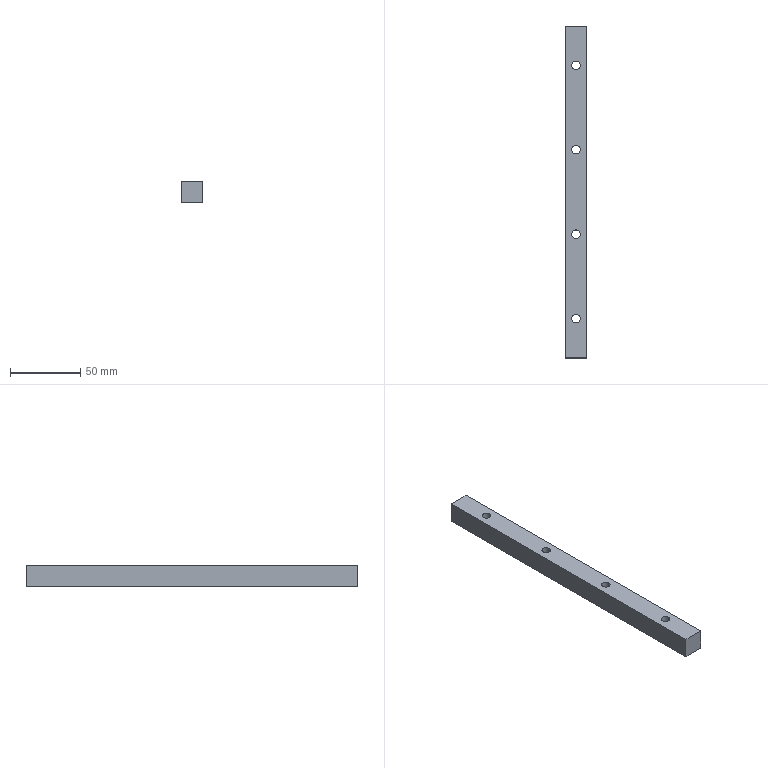Part | 1 solid | 14 faces | box 15 x 236 x 15 mm | volume 51404 mm3 | cylinder 8 | plane 6 | commonest cylinder face diameters 6 x8
STEP:
#1=CARTESIAN_POINT('',(-3.,208.,-7.5));
#2=VERTEX_POINT('',#1);
#3=CARTESIAN_POINT('',(3.,208.,-7.5));
#4=VERTEX_POINT('',#3);
#5=CARTESIAN_POINT('',(0.,208.,-7.5));
#6=DIRECTION('',(0.,0.,1.));
#7=DIRECTION('',(1.,0.,0.));
#8=AXIS2_PLACEMENT_3D('',#5,#6,#7);
#9=CIRCLE('',#8,3.);
#10=EDGE_CURVE('',#2,#4,#9,.T.);
#11=ORIENTED_EDGE('',*,*,#10,.F.);
#12=CARTESIAN_POINT('',(-3.,208.,7.5));
#13=VERTEX_POINT('',#12);
#14=CARTESIAN_POINT('',(-3.,208.,7.5));
#15=DIRECTION('',(0.,0.,1.));
#16=VECTOR('',#15,1000.);
#17=LINE('',#14,#16);
#18=EDGE_CURVE('',#2,#13,#17,.T.);
#19=ORIENTED_EDGE('',*,*,#18,.T.);
#20=CARTESIAN_POINT('',(3.,208.,7.5));
#21=VERTEX_POINT('',#20);
#22=CARTESIAN_POINT('',(0.,208.,7.5));
#23=DIRECTION('',(0.,0.,1.));
#24=DIRECTION('',(1.,0.,0.));
#25=AXIS2_PLACEMENT_3D('',#22,#23,#24);
#26=CIRCLE('',#25,3.);
#27=EDGE_CURVE('',#13,#21,#26,.T.);
#28=ORIENTED_EDGE('',*,*,#27,.T.);
#29=CARTESIAN_POINT('',(3.,208.,7.5));
#30=DIRECTION('',(0.,0.,1.));
#31=VECTOR('',#30,1000.);
#32=LINE('',#29,#31);
#33=EDGE_CURVE('',#4,#21,#32,.T.);
#34=ORIENTED_EDGE('',*,*,#33,.F.);
#35=EDGE_LOOP('',(#11,#19,#28,#34));
#36=FACE_OUTER_BOUND('',#35,.T.);
#37=CARTESIAN_POINT('',(0.,208.,7.5));
#38=DIRECTION('',(0.,0.,1.));
#39=DIRECTION('',(1.,0.,0.));
#40=AXIS2_PLACEMENT_3D('',#37,#38,#39);
#41=CYLINDRICAL_SURFACE('',#40,3.);
#42=ADVANCED_FACE('',(#36),#41,.F.);
#43=CARTESIAN_POINT('',(-3.,148.,-7.5));
#44=VERTEX_POINT('',#43);
#45=CARTESIAN_POINT('',(3.,148.,-7.5));
#46=VERTEX_POINT('',#45);
#47=CARTESIAN_POINT('',(0.,148.,-7.5));
#48=DIRECTION('',(0.,0.,1.));
#49=DIRECTION('',(1.,0.,0.));
#50=AXIS2_PLACEMENT_3D('',#47,#48,#49);
#51=CIRCLE('',#50,3.);
#52=EDGE_CURVE('',#44,#46,#51,.T.);
#53=ORIENTED_EDGE('',*,*,#52,.F.);
#54=CARTESIAN_POINT('',(-3.,148.,7.5));
#55=VERTEX_POINT('',#54);
#56=CARTESIAN_POINT('',(-3.,148.,7.5));
#57=DIRECTION('',(0.,0.,1.));
#58=VECTOR('',#57,1000.);
#59=LINE('',#56,#58);
#60=EDGE_CURVE('',#44,#55,#59,.T.);
#61=ORIENTED_EDGE('',*,*,#60,.T.);
#62=CARTESIAN_POINT('',(3.,148.,7.5));
#63=VERTEX_POINT('',#62);
#64=CARTESIAN_POINT('',(0.,148.,7.5));
#65=DIRECTION('',(0.,0.,1.));
#66=DIRECTION('',(1.,0.,0.));
#67=AXIS2_PLACEMENT_3D('',#64,#65,#66);
#68=CIRCLE('',#67,3.);
#69=EDGE_CURVE('',#55,#63,#68,.T.);
#70=ORIENTED_EDGE('',*,*,#69,.T.);
#71=CARTESIAN_POINT('',(3.,148.,7.5));
#72=DIRECTION('',(0.,0.,1.));
#73=VECTOR('',#72,1000.);
#74=LINE('',#71,#73);
#75=EDGE_CURVE('',#46,#63,#74,.T.);
#76=ORIENTED_EDGE('',*,*,#75,.F.);
#77=EDGE_LOOP('',(#53,#61,#70,#76));
#78=FACE_OUTER_BOUND('',#77,.T.);
#79=CARTESIAN_POINT('',(0.,148.,7.5));
#80=DIRECTION('',(0.,0.,1.));
#81=DIRECTION('',(1.,0.,0.));
#82=AXIS2_PLACEMENT_3D('',#79,#80,#81);
#83=CYLINDRICAL_SURFACE('',#82,3.);
#84=ADVANCED_FACE('',(#78),#83,.F.);
#85=CARTESIAN_POINT('',(-3.,88.,-7.5));
#86=VERTEX_POINT('',#85);
#87=CARTESIAN_POINT('',(3.,88.,-7.5));
#88=VERTEX_POINT('',#87);
#89=CARTESIAN_POINT('',(0.,88.,-7.5));
#90=DIRECTION('',(0.,0.,1.));
#91=DIRECTION('',(1.,0.,0.));
#92=AXIS2_PLACEMENT_3D('',#89,#90,#91);
#93=CIRCLE('',#92,3.);
#94=EDGE_CURVE('',#86,#88,#93,.T.);
#95=ORIENTED_EDGE('',*,*,#94,.F.);
#96=CARTESIAN_POINT('',(-3.,88.,7.5));
#97=VERTEX_POINT('',#96);
#98=CARTESIAN_POINT('',(-3.,88.,7.5));
#99=DIRECTION('',(0.,0.,1.));
#100=VECTOR('',#99,1000.);
#101=LINE('',#98,#100);
#102=EDGE_CURVE('',#86,#97,#101,.T.);
#103=ORIENTED_EDGE('',*,*,#102,.T.);
#104=CARTESIAN_POINT('',(3.,88.,7.5));
#105=VERTEX_POINT('',#104);
#106=CARTESIAN_POINT('',(0.,88.,7.5));
#107=DIRECTION('',(0.,0.,1.));
#108=DIRECTION('',(1.,0.,0.));
#109=AXIS2_PLACEMENT_3D('',#106,#107,#108);
#110=CIRCLE('',#109,3.);
#111=EDGE_CURVE('',#97,#105,#110,.T.);
#112=ORIENTED_EDGE('',*,*,#111,.T.);
#113=CARTESIAN_POINT('',(3.,88.,7.5));
#114=DIRECTION('',(0.,0.,1.));
#115=VECTOR('',#114,1000.);
#116=LINE('',#113,#115);
#117=EDGE_CURVE('',#88,#105,#116,.T.);
#118=ORIENTED_EDGE('',*,*,#117,.F.);
#119=EDGE_LOOP('',(#95,#103,#112,#118));
#120=FACE_OUTER_BOUND('',#119,.T.);
#121=CARTESIAN_POINT('',(0.,88.,7.5));
#122=DIRECTION('',(0.,0.,1.));
#123=DIRECTION('',(1.,0.,0.));
#124=AXIS2_PLACEMENT_3D('',#121,#122,#123);
#125=CYLINDRICAL_SURFACE('',#124,3.);
#126=ADVANCED_FACE('',(#120),#125,.F.);
#127=CARTESIAN_POINT('',(-3.,28.,-7.5));
#128=VERTEX_POINT('',#127);
#129=CARTESIAN_POINT('',(3.,28.,-7.5));
#130=VERTEX_POINT('',#129);
#131=CARTESIAN_POINT('',(0.,28.,-7.5));
#132=DIRECTION('',(0.,0.,1.));
#133=DIRECTION('',(1.,0.,0.));
#134=AXIS2_PLACEMENT_3D('',#131,#132,#133);
#135=CIRCLE('',#134,3.);
#136=EDGE_CURVE('',#128,#130,#135,.T.);
#137=ORIENTED_EDGE('',*,*,#136,.F.);
#138=CARTESIAN_POINT('',(-3.,28.,7.5));
#139=VERTEX_POINT('',#138);
#140=CARTESIAN_POINT('',(-3.,28.,7.5));
#141=DIRECTION('',(0.,0.,1.));
#142=VECTOR('',#141,1000.);
#143=LINE('',#140,#142);
#144=EDGE_CURVE('',#128,#139,#143,.T.);
#145=ORIENTED_EDGE('',*,*,#144,.T.);
#146=CARTESIAN_POINT('',(3.,28.,7.5));
#147=VERTEX_POINT('',#146);
#148=CARTESIAN_POINT('',(0.,28.,7.5));
#149=DIRECTION('',(0.,0.,1.));
#150=DIRECTION('',(1.,0.,0.));
#151=AXIS2_PLACEMENT_3D('',#148,#149,#150);
#152=CIRCLE('',#151,3.);
#153=EDGE_CURVE('',#139,#147,#152,.T.);
#154=ORIENTED_EDGE('',*,*,#153,.T.);
#155=CARTESIAN_POINT('',(3.,28.,7.5));
#156=DIRECTION('',(0.,0.,1.));
#157=VECTOR('',#156,1000.);
#158=LINE('',#155,#157);
#159=EDGE_CURVE('',#130,#147,#158,.T.);
#160=ORIENTED_EDGE('',*,*,#159,.F.);
#161=EDGE_LOOP('',(#137,#145,#154,#160));
#162=FACE_OUTER_BOUND('',#161,.T.);
#163=CARTESIAN_POINT('',(0.,28.,7.5));
#164=DIRECTION('',(0.,0.,1.));
#165=DIRECTION('',(1.,0.,0.));
#166=AXIS2_PLACEMENT_3D('',#163,#164,#165);
#167=CYLINDRICAL_SURFACE('',#166,3.);
#168=ADVANCED_FACE('',(#162),#167,.F.);
#169=CARTESIAN_POINT('',(0.,208.,7.5));
#170=DIRECTION('',(0.,0.,1.));
#171=DIRECTION('',(1.,0.,0.));
#172=AXIS2_PLACEMENT_3D('',#169,#170,#171);
#173=CIRCLE('',#172,3.);
#174=EDGE_CURVE('',#21,#13,#173,.T.);
#175=ORIENTED_EDGE('',*,*,#174,.F.);
#176=ORIENTED_EDGE('',*,*,#27,.F.);
#177=EDGE_LOOP('',(#175,#176));
#178=FACE_BOUND('',#177,.T.);
#179=CARTESIAN_POINT('',(0.,148.,7.5));
#180=DIRECTION('',(0.,0.,1.));
#181=DIRECTION('',(1.,0.,0.));
#182=AXIS2_PLACEMENT_3D('',#179,#180,#181);
#183=CIRCLE('',#182,3.);
#184=EDGE_CURVE('',#63,#55,#183,.T.);
#185=ORIENTED_EDGE('',*,*,#184,.F.);
#186=ORIENTED_EDGE('',*,*,#69,.F.);
#187=EDGE_LOOP('',(#185,#186));
#188=FACE_BOUND('',#187,.T.);
#189=CARTESIAN_POINT('',(0.,88.,7.5));
#190=DIRECTION('',(0.,0.,1.));
#191=DIRECTION('',(1.,0.,0.));
#192=AXIS2_PLACEMENT_3D('',#189,#190,#191);
#193=CIRCLE('',#192,3.);
#194=EDGE_CURVE('',#105,#97,#193,.T.);
#195=ORIENTED_EDGE('',*,*,#194,.F.);
#196=ORIENTED_EDGE('',*,*,#111,.F.);
#197=EDGE_LOOP('',(#195,#196));
#198=FACE_BOUND('',#197,.T.);
#199=CARTESIAN_POINT('',(-7.5,0.,7.5));
#200=VERTEX_POINT('',#199);
#201=CARTESIAN_POINT('',(7.5,0.,7.5));
#202=VERTEX_POINT('',#201);
#203=CARTESIAN_POINT('',(-7.5,0.,7.5));
#204=DIRECTION('',(1.,0.,0.));
#205=VECTOR('',#204,1000.);
#206=LINE('',#203,#205);
#207=EDGE_CURVE('',#200,#202,#206,.T.);
#208=ORIENTED_EDGE('',*,*,#207,.T.);
#209=CARTESIAN_POINT('',(7.5,236.,7.5));
#210=VERTEX_POINT('',#209);
#211=CARTESIAN_POINT('',(7.5,236.,7.5));
#212=DIRECTION('',(0.,-1.,0.));
#213=VECTOR('',#212,1000.);
#214=LINE('',#211,#213);
#215=EDGE_CURVE('',#210,#202,#214,.T.);
#216=ORIENTED_EDGE('',*,*,#215,.F.);
#217=CARTESIAN_POINT('',(-7.5,236.,7.5));
#218=VERTEX_POINT('',#217);
#219=CARTESIAN_POINT('',(-7.5,236.,7.5));
#220=DIRECTION('',(1.,0.,0.));
#221=VECTOR('',#220,1000.);
#222=LINE('',#219,#221);
#223=EDGE_CURVE('',#218,#210,#222,.T.);
#224=ORIENTED_EDGE('',*,*,#223,.F.);
#225=CARTESIAN_POINT('',(-7.5,236.,7.5));
#226=DIRECTION('',(0.,-1.,0.));
#227=VECTOR('',#226,1000.);
#228=LINE('',#225,#227);
#229=EDGE_CURVE('',#218,#200,#228,.T.);
#230=ORIENTED_EDGE('',*,*,#229,.T.);
#231=EDGE_LOOP('',(#208,#216,#224,#230));
#232=FACE_OUTER_BOUND('',#231,.T.);
#233=CARTESIAN_POINT('',(0.,28.,7.5));
#234=DIRECTION('',(0.,0.,1.));
#235=DIRECTION('',(1.,0.,0.));
#236=AXIS2_PLACEMENT_3D('',#233,#234,#235);
#237=CIRCLE('',#236,3.);
#238=EDGE_CURVE('',#147,#139,#237,.T.);
#239=ORIENTED_EDGE('',*,*,#238,.F.);
#240=ORIENTED_EDGE('',*,*,#153,.F.);
#241=EDGE_LOOP('',(#239,#240));
#242=FACE_BOUND('',#241,.T.);
#243=CARTESIAN_POINT('',(-7.5,236.,7.5));
#244=DIRECTION('',(0.,0.,-1.));
#245=DIRECTION('',(-1.,0.,0.));
#246=AXIS2_PLACEMENT_3D('',#243,#244,#245);
#247=PLANE('',#246);
#248=ADVANCED_FACE('',(#178,#188,#198,#232,#242),#247,.F.);
#249=CARTESIAN_POINT('',(7.5,0.,-7.5));
#250=VERTEX_POINT('',#249);
#251=CARTESIAN_POINT('',(7.5,0.,7.5));
#252=DIRECTION('',(0.,0.,-1.));
#253=VECTOR('',#252,1000.);
#254=LINE('',#251,#253);
#255=EDGE_CURVE('',#202,#250,#254,.T.);
#256=ORIENTED_EDGE('',*,*,#255,.T.);
#257=CARTESIAN_POINT('',(7.5,236.,-7.5));
#258=VERTEX_POINT('',#257);
#259=CARTESIAN_POINT('',(7.5,236.,-7.5));
#260=DIRECTION('',(0.,-1.,0.));
#261=VECTOR('',#260,1000.);
#262=LINE('',#259,#261);
#263=EDGE_CURVE('',#258,#250,#262,.T.);
#264=ORIENTED_EDGE('',*,*,#263,.F.);
#265=CARTESIAN_POINT('',(7.5,236.,7.5));
#266=DIRECTION('',(0.,0.,-1.));
#267=VECTOR('',#266,1000.);
#268=LINE('',#265,#267);
#269=EDGE_CURVE('',#210,#258,#268,.T.);
#270=ORIENTED_EDGE('',*,*,#269,.F.);
#271=ORIENTED_EDGE('',*,*,#215,.T.);
#272=EDGE_LOOP('',(#256,#264,#270,#271));
#273=FACE_OUTER_BOUND('',#272,.T.);
#274=CARTESIAN_POINT('',(7.5,236.,7.5));
#275=DIRECTION('',(-1.,0.,0.));
#276=DIRECTION('',(0.,0.,1.));
#277=AXIS2_PLACEMENT_3D('',#274,#275,#276);
#278=PLANE('',#277);
#279=ADVANCED_FACE('',(#273),#278,.F.);
#280=CARTESIAN_POINT('',(0.,208.,-7.5));
#281=DIRECTION('',(0.,0.,1.));
#282=DIRECTION('',(1.,0.,0.));
#283=AXIS2_PLACEMENT_3D('',#280,#281,#282);
#284=CIRCLE('',#283,3.);
#285=EDGE_CURVE('',#4,#2,#284,.T.);
#286=ORIENTED_EDGE('',*,*,#285,.T.);
#287=ORIENTED_EDGE('',*,*,#10,.T.);
#288=EDGE_LOOP('',(#286,#287));
#289=FACE_BOUND('',#288,.T.);
#290=CARTESIAN_POINT('',(0.,148.,-7.5));
#291=DIRECTION('',(0.,0.,1.));
#292=DIRECTION('',(1.,0.,0.));
#293=AXIS2_PLACEMENT_3D('',#290,#291,#292);
#294=CIRCLE('',#293,3.);
#295=EDGE_CURVE('',#46,#44,#294,.T.);
#296=ORIENTED_EDGE('',*,*,#295,.T.);
#297=ORIENTED_EDGE('',*,*,#52,.T.);
#298=EDGE_LOOP('',(#296,#297));
#299=FACE_BOUND('',#298,.T.);
#300=CARTESIAN_POINT('',(0.,88.,-7.5));
#301=DIRECTION('',(0.,0.,1.));
#302=DIRECTION('',(1.,0.,0.));
#303=AXIS2_PLACEMENT_3D('',#300,#301,#302);
#304=CIRCLE('',#303,3.);
#305=EDGE_CURVE('',#88,#86,#304,.T.);
#306=ORIENTED_EDGE('',*,*,#305,.T.);
#307=ORIENTED_EDGE('',*,*,#94,.T.);
#308=EDGE_LOOP('',(#306,#307));
#309=FACE_BOUND('',#308,.T.);
#310=CARTESIAN_POINT('',(0.,28.,-7.5));
#311=DIRECTION('',(0.,0.,1.));
#312=DIRECTION('',(1.,0.,0.));
#313=AXIS2_PLACEMENT_3D('',#310,#311,#312);
#314=CIRCLE('',#313,3.);
#315=EDGE_CURVE('',#130,#128,#314,.T.);
#316=ORIENTED_EDGE('',*,*,#315,.T.);
#317=ORIENTED_EDGE('',*,*,#136,.T.);
#318=EDGE_LOOP('',(#316,#317));
#319=FACE_BOUND('',#318,.T.);
#320=CARTESIAN_POINT('',(-7.5,0.,-7.5));
#321=VERTEX_POINT('',#320);
#322=CARTESIAN_POINT('',(-7.5,0.,-7.5));
#323=DIRECTION('',(-1.,0.,0.));
#324=VECTOR('',#323,1000.);
#325=LINE('',#322,#324);
#326=EDGE_CURVE('',#250,#321,#325,.T.);
#327=ORIENTED_EDGE('',*,*,#326,.T.);
#328=CARTESIAN_POINT('',(-7.5,236.,-7.5));
#329=VERTEX_POINT('',#328);
#330=CARTESIAN_POINT('',(-7.5,236.,-7.5));
#331=DIRECTION('',(0.,-1.,0.));
#332=VECTOR('',#331,1000.);
#333=LINE('',#330,#332);
#334=EDGE_CURVE('',#329,#321,#333,.T.);
#335=ORIENTED_EDGE('',*,*,#334,.F.);
#336=CARTESIAN_POINT('',(-7.5,236.,-7.5));
#337=DIRECTION('',(-1.,0.,0.));
#338=VECTOR('',#337,1000.);
#339=LINE('',#336,#338);
#340=EDGE_CURVE('',#258,#329,#339,.T.);
#341=ORIENTED_EDGE('',*,*,#340,.F.);
#342=ORIENTED_EDGE('',*,*,#263,.T.);
#343=EDGE_LOOP('',(#327,#335,#341,#342));
#344=FACE_OUTER_BOUND('',#343,.T.);
#345=CARTESIAN_POINT('',(-7.5,236.,-7.5));
#346=DIRECTION('',(0.,0.,1.));
#347=DIRECTION('',(1.,0.,0.));
#348=AXIS2_PLACEMENT_3D('',#345,#346,#347);
#349=PLANE('',#348);
#350=ADVANCED_FACE('',(#289,#299,#309,#319,#344),#349,.F.);
#351=CARTESIAN_POINT('',(-7.5,0.,7.5));
#352=DIRECTION('',(0.,0.,1.));
#353=VECTOR('',#352,1000.);
#354=LINE('',#351,#353);
#355=EDGE_CURVE('',#321,#200,#354,.T.);
#356=ORIENTED_EDGE('',*,*,#355,.T.);
#357=ORIENTED_EDGE('',*,*,#229,.F.);
#358=CARTESIAN_POINT('',(-7.5,236.,7.5));
#359=DIRECTION('',(0.,0.,1.));
#360=VECTOR('',#359,1000.);
#361=LINE('',#358,#360);
#362=EDGE_CURVE('',#329,#218,#361,.T.);
#363=ORIENTED_EDGE('',*,*,#362,.F.);
#364=ORIENTED_EDGE('',*,*,#334,.T.);
#365=EDGE_LOOP('',(#356,#357,#363,#364));
#366=FACE_OUTER_BOUND('',#365,.T.);
#367=CARTESIAN_POINT('',(-7.5,236.,7.5));
#368=DIRECTION('',(1.,0.,0.));
#369=DIRECTION('',(0.,0.,-1.));
#370=AXIS2_PLACEMENT_3D('',#367,#368,#369);
#371=PLANE('',#370);
#372=ADVANCED_FACE('',(#366),#371,.F.);
#373=ORIENTED_EDGE('',*,*,#269,.T.);
#374=ORIENTED_EDGE('',*,*,#340,.T.);
#375=ORIENTED_EDGE('',*,*,#362,.T.);
#376=ORIENTED_EDGE('',*,*,#223,.T.);
#377=EDGE_LOOP('',(#373,#374,#375,#376));
#378=FACE_OUTER_BOUND('',#377,.T.);
#379=CARTESIAN_POINT('',(0.,236.,0.));
#380=DIRECTION('',(0.,-1.,0.));
#381=DIRECTION('',(0.,0.,-1.));
#382=AXIS2_PLACEMENT_3D('',#379,#380,#381);
#383=PLANE('',#382);
#384=ADVANCED_FACE('',(#378),#383,.F.);
#385=ORIENTED_EDGE('',*,*,#255,.F.);
#386=ORIENTED_EDGE('',*,*,#207,.F.);
#387=ORIENTED_EDGE('',*,*,#355,.F.);
#388=ORIENTED_EDGE('',*,*,#326,.F.);
#389=EDGE_LOOP('',(#385,#386,#387,#388));
#390=FACE_OUTER_BOUND('',#389,.T.);
#391=CARTESIAN_POINT('',(0.,0.,0.));
#392=DIRECTION('',(0.,-1.,0.));
#393=DIRECTION('',(0.,0.,-1.));
#394=AXIS2_PLACEMENT_3D('',#391,#392,#393);
#395=PLANE('',#394);
#396=ADVANCED_FACE('',(#390),#395,.T.);
#397=ORIENTED_EDGE('',*,*,#144,.F.);
#398=ORIENTED_EDGE('',*,*,#315,.F.);
#399=ORIENTED_EDGE('',*,*,#159,.T.);
#400=ORIENTED_EDGE('',*,*,#238,.T.);
#401=EDGE_LOOP('',(#397,#398,#399,#400));
#402=FACE_OUTER_BOUND('',#401,.T.);
#403=CARTESIAN_POINT('',(0.,28.,7.5));
#404=DIRECTION('',(0.,0.,1.));
#405=DIRECTION('',(1.,0.,0.));
#406=AXIS2_PLACEMENT_3D('',#403,#404,#405);
#407=CYLINDRICAL_SURFACE('',#406,3.);
#408=ADVANCED_FACE('',(#402),#407,.F.);
#409=ORIENTED_EDGE('',*,*,#102,.F.);
#410=ORIENTED_EDGE('',*,*,#305,.F.);
#411=ORIENTED_EDGE('',*,*,#117,.T.);
#412=ORIENTED_EDGE('',*,*,#194,.T.);
#413=EDGE_LOOP('',(#409,#410,#411,#412));
#414=FACE_OUTER_BOUND('',#413,.T.);
#415=CARTESIAN_POINT('',(0.,88.,7.5));
#416=DIRECTION('',(0.,0.,1.));
#417=DIRECTION('',(1.,0.,0.));
#418=AXIS2_PLACEMENT_3D('',#415,#416,#417);
#419=CYLINDRICAL_SURFACE('',#418,3.);
#420=ADVANCED_FACE('',(#414),#419,.F.);
#421=ORIENTED_EDGE('',*,*,#60,.F.);
#422=ORIENTED_EDGE('',*,*,#295,.F.);
#423=ORIENTED_EDGE('',*,*,#75,.T.);
#424=ORIENTED_EDGE('',*,*,#184,.T.);
#425=EDGE_LOOP('',(#421,#422,#423,#424));
#426=FACE_OUTER_BOUND('',#425,.T.);
#427=CARTESIAN_POINT('',(0.,148.,7.5));
#428=DIRECTION('',(0.,0.,1.));
#429=DIRECTION('',(1.,0.,0.));
#430=AXIS2_PLACEMENT_3D('',#427,#428,#429);
#431=CYLINDRICAL_SURFACE('',#430,3.);
#432=ADVANCED_FACE('',(#426),#431,.F.);
#433=ORIENTED_EDGE('',*,*,#18,.F.);
#434=ORIENTED_EDGE('',*,*,#285,.F.);
#435=ORIENTED_EDGE('',*,*,#33,.T.);
#436=ORIENTED_EDGE('',*,*,#174,.T.);
#437=EDGE_LOOP('',(#433,#434,#435,#436));
#438=FACE_OUTER_BOUND('',#437,.T.);
#439=CARTESIAN_POINT('',(0.,208.,7.5));
#440=DIRECTION('',(0.,0.,1.));
#441=DIRECTION('',(1.,0.,0.));
#442=AXIS2_PLACEMENT_3D('',#439,#440,#441);
#443=CYLINDRICAL_SURFACE('',#442,3.);
#444=ADVANCED_FACE('',(#438),#443,.F.);
#445=CLOSED_SHELL('',(#42,#84,#126,#168,#248,#279,#350,#372,#384,#396,#408,#420,#432,#444));
#446=MANIFOLD_SOLID_BREP('',#445);
#447=CARTESIAN_POINT('',(0.,0.,0.));
#448=DIRECTION('',(0.,0.,1.));
#449=DIRECTION('',(1.,0.,0.));
#450=AXIS2_PLACEMENT_3D('',#447,#448,#449);
#451=(LENGTH_UNIT()NAMED_UNIT(*)SI_UNIT(.MILLI.,.METRE.));
#452=UNCERTAINTY_MEASURE_WITH_UNIT(LENGTH_MEASURE(0.00001),#451,'','');
#453=(NAMED_UNIT(*)PLANE_ANGLE_UNIT()SI_UNIT($,.RADIAN.));
#454=(NAMED_UNIT(*)SI_UNIT($,.STERADIAN.)SOLID_ANGLE_UNIT());
#455=(GEOMETRIC_REPRESENTATION_CONTEXT(3)GLOBAL_UNCERTAINTY_ASSIGNED_CONTEXT((#452))GLOBAL_UNIT_ASSIGNED_CONTEXT((#451,#453,#454))REPRESENTATION_CONTEXT('',''));
#456=ADVANCED_BREP_SHAPE_REPRESENTATION('',(#446,#450),#455);